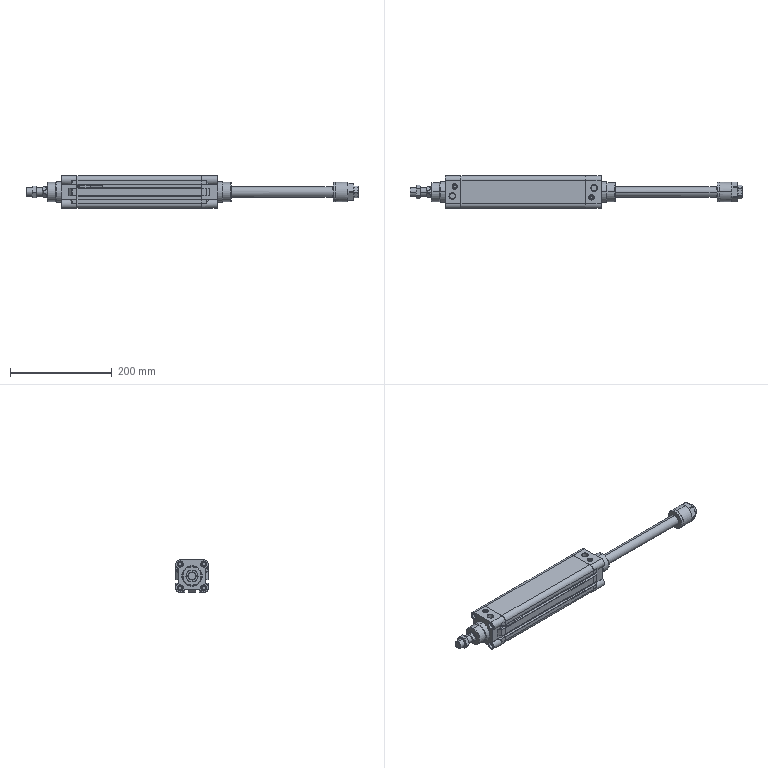Part | STEP file | SEJ50x200-20S_0020_+_DMSE-2_ | 7 solids | 587 faces | box 651 x 64.6 x 64 mm | volume 961135 mm3 | plane 261 | cylinder 224 | cone 96 | torus 6 | commonest cylinder face diameters 1 x102 6.647 x16 12.4 x16 17.5 x10 19 x10 3 x8